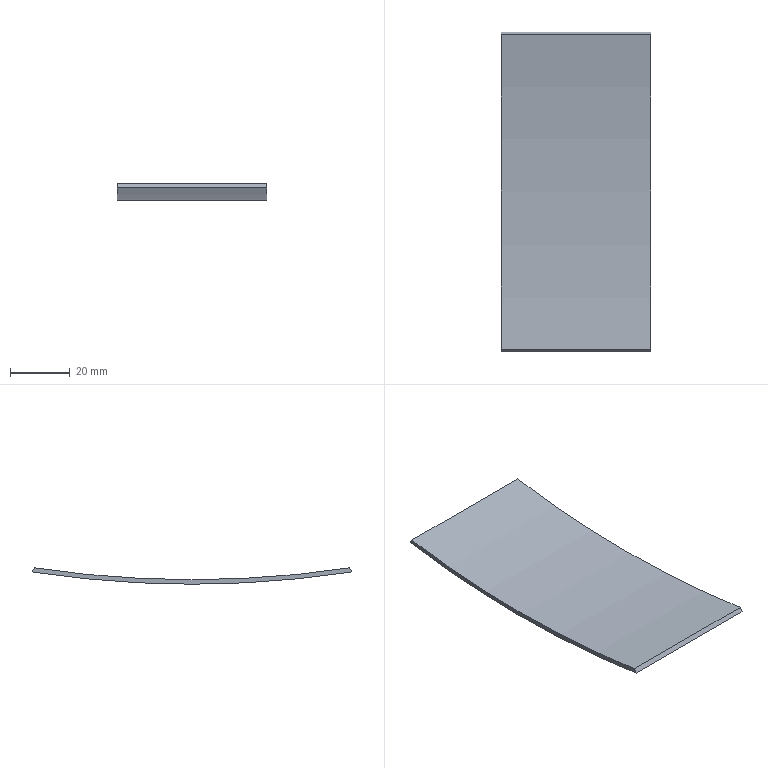Part | STEP file | 1 solid | 6 faces | box 50 x 106.693 x 5.46 mm | volume 7969 mm3 | plane 4 | cylinder 2 | commonest cylinder face diameters 700 x1 703 x1
STEP:
#1=CARTESIAN_POINT('',(0.,0.,0.));
#2=DIRECTION('',(0.,0.,1.));
#3=DIRECTION('',(1.,0.,0.));
#4=AXIS2_PLACEMENT_3D('',#1,#2,#3);
#5=CARTESIAN_POINT('',(25.,53.346,-347.428));
#6=VERTEX_POINT('',#5);
#7=CARTESIAN_POINT('',(25.,-53.346,-347.428));
#8=VERTEX_POINT('',#7);
#9=CARTESIAN_POINT('',(25.,0.,0.));
#10=DIRECTION('',(-1.,0.,0.));
#11=DIRECTION('',(0.,0.,-1.));
#12=AXIS2_PLACEMENT_3D('',#9,#10,#11);
#13=CIRCLE('',#12,351.5);
#14=CARTESIAN_POINT('',(-25.,0.,0.));
#15=DIRECTION('',(1.,0.,0.));
#16=DIRECTION('',(0.,0.,-1.));
#17=AXIS2_PLACEMENT_3D('',#14,#15,#16);
#18=CYLINDRICAL_SURFACE('',#17,351.5);
#19=CARTESIAN_POINT('',(6.283,50.));
#20=DIRECTION('',(-1.,0.));
#21=VECTOR('',#20,1.);
#22=LINE('',#19,#21);
#23=(GEOMETRIC_REPRESENTATION_CONTEXT(2)PARAMETRIC_REPRESENTATION_CONTEXT()REPRESENTATION_CONTEXT('',''));
#24=DEFINITIONAL_REPRESENTATION('',(#22),#23);
#25=PCURVE('',#18,#24);
#26=CARTESIAN_POINT('',(25.,-69.931,-393.84));
#27=DIRECTION('',(1.,0.,0.));
#28=DIRECTION('',(0.,0.,-1.));
#29=AXIS2_PLACEMENT_3D('',#26,#27,#28);
#30=PLANE('',#29);
#31=CARTESIAN_POINT('',(-42.34,69.931));
#32=CARTESIAN_POINT('',(-42.34,-538.885));
#33=CARTESIAN_POINT('',(-569.59,-234.477));
#34=CARTESIAN_POINT('',(-1096.84,69.931));
#35=CARTESIAN_POINT('',(-569.59,374.339));
#36=CARTESIAN_POINT('',(-42.34,678.747));
#37=CARTESIAN_POINT('',(-42.34,69.931));
#38=(BOUNDED_CURVE()B_SPLINE_CURVE(2,(#31,#32,#33,#34,#35,#36,#37),.UNSPECIFIED.,.T.,.F.)B_SPLINE_CURVE_WITH_KNOTS((1,2,2,2,2,1),(-2.094,0.,2.094,4.189,6.283,8.378),.UNSPECIFIED.)CURVE()GEOMETRIC_REPRESENTATION_ITEM()RATIONAL_B_SPLINE_CURVE((1.,0.5,1.,0.5,1.,0.5,1.))REPRESENTATION_ITEM(''));
#39=(GEOMETRIC_REPRESENTATION_CONTEXT(2)PARAMETRIC_REPRESENTATION_CONTEXT()REPRESENTATION_CONTEXT('',''));
#40=DEFINITIONAL_REPRESENTATION('',(#38),#39);
#41=PCURVE('',#30,#40);
#42=SURFACE_CURVE('',#13,(#25,#41),.PCURVE_S1.);
#43=EDGE_CURVE('',#6,#8,#42,.T.);
#44=ORIENTED_EDGE('',*,*,#43,.T.);
#45=CARTESIAN_POINT('',(-25.,-53.346,-347.428));
#46=VERTEX_POINT('',#45);
#47=CARTESIAN_POINT('',(-25.,-53.346,-347.428));
#48=DIRECTION('',(-1.,0.,0.));
#49=VECTOR('',#48,1.);
#50=LINE('',#47,#49);
#51=CARTESIAN_POINT('',(-0.1524,0.));
#52=DIRECTION('',(0.,-1.));
#53=VECTOR('',#52,1.);
#54=LINE('',#51,#53);
#55=(GEOMETRIC_REPRESENTATION_CONTEXT(2)PARAMETRIC_REPRESENTATION_CONTEXT()REPRESENTATION_CONTEXT('',''));
#56=DEFINITIONAL_REPRESENTATION('',(#54),#55);
#57=PCURVE('',#18,#56);
#58=CARTESIAN_POINT('',(-25.,-52.5,-346.04));
#59=DIRECTION('',(0.,0.8538,-0.5206));
#60=DIRECTION('',(0.,0.5206,0.8538));
#61=AXIS2_PLACEMENT_3D('',#58,#59,#60);
#62=PLANE('',#61);
#63=CARTESIAN_POINT('',(-1.626,0.));
#64=DIRECTION('',(0.,-1.));
#65=VECTOR('',#64,1.);
#66=LINE('',#63,#65);
#67=(GEOMETRIC_REPRESENTATION_CONTEXT(2)PARAMETRIC_REPRESENTATION_CONTEXT()REPRESENTATION_CONTEXT('',''));
#68=DEFINITIONAL_REPRESENTATION('',(#66),#67);
#69=PCURVE('',#62,#68);
#70=SURFACE_CURVE('',#50,(#57,#69),.PCURVE_S1.);
#71=EDGE_CURVE('',#8,#46,#70,.T.);
#72=ORIENTED_EDGE('',*,*,#71,.T.);
#73=CARTESIAN_POINT('',(-25.,53.346,-347.428));
#74=VERTEX_POINT('',#73);
#75=CARTESIAN_POINT('',(-25.,0.,0.));
#76=DIRECTION('',(1.,0.,0.));
#77=DIRECTION('',(0.,0.,-1.));
#78=AXIS2_PLACEMENT_3D('',#75,#76,#77);
#79=CIRCLE('',#78,351.5);
#80=CARTESIAN_POINT('',(-6.283,0.));
#81=DIRECTION('',(1.,0.));
#82=VECTOR('',#81,1.);
#83=LINE('',#80,#82);
#84=(GEOMETRIC_REPRESENTATION_CONTEXT(2)PARAMETRIC_REPRESENTATION_CONTEXT()REPRESENTATION_CONTEXT('',''));
#85=DEFINITIONAL_REPRESENTATION('',(#83),#84);
#86=PCURVE('',#18,#85);
#87=CARTESIAN_POINT('',(-25.,0.,0.));
#88=DIRECTION('',(-1.,0.,0.));
#89=DIRECTION('',(0.,0.,1.));
#90=AXIS2_PLACEMENT_3D('',#87,#88,#89);
#91=PLANE('',#90);
#92=CARTESIAN_POINT('',(-351.5,0.));
#93=CARTESIAN_POINT('',(-351.5,608.816));
#94=CARTESIAN_POINT('',(175.75,304.408));
#95=CARTESIAN_POINT('',(703.,0.));
#96=CARTESIAN_POINT('',(175.75,-304.408));
#97=CARTESIAN_POINT('',(-351.5,-608.816));
#98=CARTESIAN_POINT('',(-351.5,0.));
#99=(BOUNDED_CURVE()B_SPLINE_CURVE(2,(#92,#93,#94,#95,#96,#97,#98),.UNSPECIFIED.,.T.,.F.)B_SPLINE_CURVE_WITH_KNOTS((1,2,2,2,2,1),(-2.094,0.,2.094,4.189,6.283,8.378),.UNSPECIFIED.)CURVE()GEOMETRIC_REPRESENTATION_ITEM()RATIONAL_B_SPLINE_CURVE((1.,0.5,1.,0.5,1.,0.5,1.))REPRESENTATION_ITEM(''));
#100=(GEOMETRIC_REPRESENTATION_CONTEXT(2)PARAMETRIC_REPRESENTATION_CONTEXT()REPRESENTATION_CONTEXT('',''));
#101=DEFINITIONAL_REPRESENTATION('',(#99),#100);
#102=PCURVE('',#91,#101);
#103=SURFACE_CURVE('',#79,(#86,#102),.PCURVE_S1.);
#104=EDGE_CURVE('',#46,#74,#103,.T.);
#105=ORIENTED_EDGE('',*,*,#104,.T.);
#106=CARTESIAN_POINT('',(-25.,53.346,-347.428));
#107=DIRECTION('',(1.,0.,0.));
#108=VECTOR('',#107,1.);
#109=LINE('',#106,#108);
#110=CARTESIAN_POINT('',(0.1524,0.));
#111=DIRECTION('',(0.,1.));
#112=VECTOR('',#111,1.);
#113=LINE('',#110,#112);
#114=(GEOMETRIC_REPRESENTATION_CONTEXT(2)PARAMETRIC_REPRESENTATION_CONTEXT()REPRESENTATION_CONTEXT('',''));
#115=DEFINITIONAL_REPRESENTATION('',(#113),#114);
#116=PCURVE('',#18,#115);
#117=CARTESIAN_POINT('',(-25.,53.346,-347.428));
#118=DIRECTION('',(0.,-0.8538,-0.5206));
#119=DIRECTION('',(0.,0.5206,-0.8538));
#120=AXIS2_PLACEMENT_3D('',#117,#118,#119);
#121=PLANE('',#120);
#122=CARTESIAN_POINT('',(0.,0.));
#123=DIRECTION('',(0.,1.));
#124=VECTOR('',#123,1.);
#125=LINE('',#122,#124);
#126=(GEOMETRIC_REPRESENTATION_CONTEXT(2)PARAMETRIC_REPRESENTATION_CONTEXT()REPRESENTATION_CONTEXT('',''));
#127=DEFINITIONAL_REPRESENTATION('',(#125),#126);
#128=PCURVE('',#121,#127);
#129=SURFACE_CURVE('',#109,(#116,#128),.PCURVE_S1.);
#130=EDGE_CURVE('',#74,#6,#129,.T.);
#131=ORIENTED_EDGE('',*,*,#130,.T.);
#132=EDGE_LOOP('',(#44,#72,#105,#131));
#133=FACE_BOUND('',#132,.T.);
#134=ADVANCED_FACE('',(#133),#18,.T.);
#135=ORIENTED_EDGE('',*,*,#71,.F.);
#136=CARTESIAN_POINT('',(25.,-52.5,-346.04));
#137=VERTEX_POINT('',#136);
#138=CARTESIAN_POINT('',(25.,-52.5,-346.04));
#139=DIRECTION('',(0.,-0.5206,-0.8538));
#140=VECTOR('',#139,1.);
#141=LINE('',#138,#140);
#142=CARTESIAN_POINT('',(0.,50.));
#143=DIRECTION('',(-1.,0.));
#144=VECTOR('',#143,1.);
#145=LINE('',#142,#144);
#146=(GEOMETRIC_REPRESENTATION_CONTEXT(2)PARAMETRIC_REPRESENTATION_CONTEXT()REPRESENTATION_CONTEXT('',''));
#147=DEFINITIONAL_REPRESENTATION('',(#145),#146);
#148=PCURVE('',#62,#147);
#149=CARTESIAN_POINT('',(-47.799,17.431));
#150=DIRECTION('',(0.8538,-0.5206));
#151=VECTOR('',#150,1.);
#152=LINE('',#149,#151);
#153=(GEOMETRIC_REPRESENTATION_CONTEXT(2)PARAMETRIC_REPRESENTATION_CONTEXT()REPRESENTATION_CONTEXT('',''));
#154=DEFINITIONAL_REPRESENTATION('',(#152),#153);
#155=PCURVE('',#30,#154);
#156=SURFACE_CURVE('',#141,(#148,#155),.PCURVE_S1.);
#157=EDGE_CURVE('',#137,#8,#156,.T.);
#158=ORIENTED_EDGE('',*,*,#157,.F.);
#159=CARTESIAN_POINT('',(-25.,-52.5,-346.04));
#160=VERTEX_POINT('',#159);
#161=CARTESIAN_POINT('',(-25.,-52.5,-346.04));
#162=DIRECTION('',(1.,0.,0.));
#163=VECTOR('',#162,1.);
#164=LINE('',#161,#163);
#165=CARTESIAN_POINT('',(0.,0.));
#166=DIRECTION('',(0.,1.));
#167=VECTOR('',#166,1.);
#168=LINE('',#165,#167);
#169=(GEOMETRIC_REPRESENTATION_CONTEXT(2)PARAMETRIC_REPRESENTATION_CONTEXT()REPRESENTATION_CONTEXT('',''));
#170=DEFINITIONAL_REPRESENTATION('',(#168),#169);
#171=PCURVE('',#62,#170);
#172=CARTESIAN_POINT('',(-25.,0.,0.));
#173=DIRECTION('',(1.,0.,0.));
#174=DIRECTION('',(0.,0.,-1.));
#175=AXIS2_PLACEMENT_3D('',#172,#173,#174);
#176=CYLINDRICAL_SURFACE('',#175,350.);
#177=CARTESIAN_POINT('',(-0.1506,0.));
#178=DIRECTION('',(0.,1.));
#179=VECTOR('',#178,1.);
#180=LINE('',#177,#179);
#181=(GEOMETRIC_REPRESENTATION_CONTEXT(2)PARAMETRIC_REPRESENTATION_CONTEXT()REPRESENTATION_CONTEXT('',''));
#182=DEFINITIONAL_REPRESENTATION('',(#180),#181);
#183=PCURVE('',#176,#182);
#184=SURFACE_CURVE('',#164,(#171,#183),.PCURVE_S1.);
#185=EDGE_CURVE('',#160,#137,#184,.T.);
#186=ORIENTED_EDGE('',*,*,#185,.F.);
#187=CARTESIAN_POINT('',(-25.,-52.5,-346.04));
#188=DIRECTION('',(0.,0.5206,0.8538));
#189=VECTOR('',#188,1.);
#190=LINE('',#187,#189);
#191=CARTESIAN_POINT('',(0.,0.));
#192=DIRECTION('',(1.,0.));
#193=VECTOR('',#192,1.);
#194=LINE('',#191,#193);
#195=(GEOMETRIC_REPRESENTATION_CONTEXT(2)PARAMETRIC_REPRESENTATION_CONTEXT()REPRESENTATION_CONTEXT('',''));
#196=DEFINITIONAL_REPRESENTATION('',(#194),#195);
#197=PCURVE('',#62,#196);
#198=CARTESIAN_POINT('',(-346.04,-52.5));
#199=DIRECTION('',(0.8538,0.5206));
#200=VECTOR('',#199,1.);
#201=LINE('',#198,#200);
#202=(GEOMETRIC_REPRESENTATION_CONTEXT(2)PARAMETRIC_REPRESENTATION_CONTEXT()REPRESENTATION_CONTEXT('',''));
#203=DEFINITIONAL_REPRESENTATION('',(#201),#202);
#204=PCURVE('',#91,#203);
#205=SURFACE_CURVE('',#190,(#197,#204),.PCURVE_S1.);
#206=EDGE_CURVE('',#46,#160,#205,.T.);
#207=ORIENTED_EDGE('',*,*,#206,.F.);
#208=EDGE_LOOP('',(#135,#158,#186,#207));
#209=FACE_BOUND('',#208,.T.);
#210=ADVANCED_FACE('',(#209),#62,.F.);
#211=ORIENTED_EDGE('',*,*,#157,.T.);
#212=ORIENTED_EDGE('',*,*,#43,.F.);
#213=CARTESIAN_POINT('',(25.,52.5,-346.04));
#214=VERTEX_POINT('',#213);
#215=CARTESIAN_POINT('',(25.,53.346,-347.428));
#216=DIRECTION('',(0.,-0.5206,0.8538));
#217=VECTOR('',#216,1.);
#218=LINE('',#215,#217);
#219=CARTESIAN_POINT('',(-46.411,123.278));
#220=DIRECTION('',(-0.8538,-0.5206));
#221=VECTOR('',#220,1.);
#222=LINE('',#219,#221);
#223=(GEOMETRIC_REPRESENTATION_CONTEXT(2)PARAMETRIC_REPRESENTATION_CONTEXT()REPRESENTATION_CONTEXT('',''));
#224=DEFINITIONAL_REPRESENTATION('',(#222),#223);
#225=PCURVE('',#30,#224);
#226=CARTESIAN_POINT('',(0.,50.));
#227=DIRECTION('',(-1.,0.));
#228=VECTOR('',#227,1.);
#229=LINE('',#226,#228);
#230=(GEOMETRIC_REPRESENTATION_CONTEXT(2)PARAMETRIC_REPRESENTATION_CONTEXT()REPRESENTATION_CONTEXT('',''));
#231=DEFINITIONAL_REPRESENTATION('',(#229),#230);
#232=PCURVE('',#121,#231);
#233=SURFACE_CURVE('',#218,(#225,#232),.PCURVE_S1.);
#234=EDGE_CURVE('',#6,#214,#233,.T.);
#235=ORIENTED_EDGE('',*,*,#234,.T.);
#236=CARTESIAN_POINT('',(25.,0.,0.));
#237=DIRECTION('',(-1.,0.,0.));
#238=DIRECTION('',(0.,0.,-1.));
#239=AXIS2_PLACEMENT_3D('',#236,#237,#238);
#240=CIRCLE('',#239,350.);
#241=CARTESIAN_POINT('',(-43.84,69.931));
#242=CARTESIAN_POINT('',(-43.84,-536.286));
#243=CARTESIAN_POINT('',(-568.84,-233.178));
#244=CARTESIAN_POINT('',(-1093.84,69.931));
#245=CARTESIAN_POINT('',(-568.84,373.04));
#246=CARTESIAN_POINT('',(-43.84,676.149));
#247=CARTESIAN_POINT('',(-43.84,69.931));
#248=(BOUNDED_CURVE()B_SPLINE_CURVE(2,(#241,#242,#243,#244,#245,#246,#247),.UNSPECIFIED.,.T.,.F.)B_SPLINE_CURVE_WITH_KNOTS((1,2,2,2,2,1),(-2.094,0.,2.094,4.189,6.283,8.378),.UNSPECIFIED.)CURVE()GEOMETRIC_REPRESENTATION_ITEM()RATIONAL_B_SPLINE_CURVE((1.,0.5,1.,0.5,1.,0.5,1.))REPRESENTATION_ITEM(''));
#249=(GEOMETRIC_REPRESENTATION_CONTEXT(2)PARAMETRIC_REPRESENTATION_CONTEXT()REPRESENTATION_CONTEXT('',''));
#250=DEFINITIONAL_REPRESENTATION('',(#248),#249);
#251=PCURVE('',#30,#250);
#252=CARTESIAN_POINT('',(6.283,50.));
#253=DIRECTION('',(-1.,0.));
#254=VECTOR('',#253,1.);
#255=LINE('',#252,#254);
#256=(GEOMETRIC_REPRESENTATION_CONTEXT(2)PARAMETRIC_REPRESENTATION_CONTEXT()REPRESENTATION_CONTEXT('',''));
#257=DEFINITIONAL_REPRESENTATION('',(#255),#256);
#258=PCURVE('',#176,#257);
#259=SURFACE_CURVE('',#240,(#251,#258),.PCURVE_S1.);
#260=EDGE_CURVE('',#214,#137,#259,.T.);
#261=ORIENTED_EDGE('',*,*,#260,.T.);
#262=EDGE_LOOP('',(#211,#212,#235,#261));
#263=FACE_BOUND('',#262,.T.);
#264=ADVANCED_FACE('',(#263),#30,.T.);
#265=CARTESIAN_POINT('',(-25.,52.5,-346.04));
#266=VERTEX_POINT('',#265);
#267=CARTESIAN_POINT('',(-25.,0.,0.));
#268=DIRECTION('',(1.,0.,0.));
#269=DIRECTION('',(0.,0.,-1.));
#270=AXIS2_PLACEMENT_3D('',#267,#268,#269);
#271=CIRCLE('',#270,350.);
#272=CARTESIAN_POINT('',(-350.,0.));
#273=CARTESIAN_POINT('',(-350.,606.218));
#274=CARTESIAN_POINT('',(175.,303.109));
#275=CARTESIAN_POINT('',(700.,0.));
#276=CARTESIAN_POINT('',(175.,-303.109));
#277=CARTESIAN_POINT('',(-350.,-606.218));
#278=CARTESIAN_POINT('',(-350.,0.));
#279=(BOUNDED_CURVE()B_SPLINE_CURVE(2,(#272,#273,#274,#275,#276,#277,#278),.UNSPECIFIED.,.T.,.F.)B_SPLINE_CURVE_WITH_KNOTS((1,2,2,2,2,1),(-2.094,0.,2.094,4.189,6.283,8.378),.UNSPECIFIED.)CURVE()GEOMETRIC_REPRESENTATION_ITEM()RATIONAL_B_SPLINE_CURVE((1.,0.5,1.,0.5,1.,0.5,1.))REPRESENTATION_ITEM(''));
#280=(GEOMETRIC_REPRESENTATION_CONTEXT(2)PARAMETRIC_REPRESENTATION_CONTEXT()REPRESENTATION_CONTEXT('',''));
#281=DEFINITIONAL_REPRESENTATION('',(#279),#280);
#282=PCURVE('',#91,#281);
#283=CARTESIAN_POINT('',(-6.283,0.));
#284=DIRECTION('',(1.,0.));
#285=VECTOR('',#284,1.);
#286=LINE('',#283,#285);
#287=(GEOMETRIC_REPRESENTATION_CONTEXT(2)PARAMETRIC_REPRESENTATION_CONTEXT()REPRESENTATION_CONTEXT('',''));
#288=DEFINITIONAL_REPRESENTATION('',(#286),#287);
#289=PCURVE('',#176,#288);
#290=SURFACE_CURVE('',#271,(#282,#289),.PCURVE_S1.);
#291=EDGE_CURVE('',#160,#266,#290,.T.);
#292=ORIENTED_EDGE('',*,*,#291,.T.);
#293=CARTESIAN_POINT('',(-25.,52.5,-346.04));
#294=DIRECTION('',(0.,0.5206,-0.8538));
#295=VECTOR('',#294,1.);
#296=LINE('',#293,#295);
#297=CARTESIAN_POINT('',(-346.04,52.5));
#298=DIRECTION('',(-0.8538,0.5206));
#299=VECTOR('',#298,1.);
#300=LINE('',#297,#299);
#301=(GEOMETRIC_REPRESENTATION_CONTEXT(2)PARAMETRIC_REPRESENTATION_CONTEXT()REPRESENTATION_CONTEXT('',''));
#302=DEFINITIONAL_REPRESENTATION('',(#300),#301);
#303=PCURVE('',#91,#302);
#304=CARTESIAN_POINT('',(-1.626,0.));
#305=DIRECTION('',(1.,0.));
#306=VECTOR('',#305,1.);
#307=LINE('',#304,#306);
#308=(GEOMETRIC_REPRESENTATION_CONTEXT(2)PARAMETRIC_REPRESENTATION_CONTEXT()REPRESENTATION_CONTEXT('',''));
#309=DEFINITIONAL_REPRESENTATION('',(#307),#308);
#310=PCURVE('',#121,#309);
#311=SURFACE_CURVE('',#296,(#303,#310),.PCURVE_S1.);
#312=EDGE_CURVE('',#266,#74,#311,.T.);
#313=ORIENTED_EDGE('',*,*,#312,.T.);
#314=ORIENTED_EDGE('',*,*,#104,.F.);
#315=ORIENTED_EDGE('',*,*,#206,.T.);
#316=EDGE_LOOP('',(#292,#313,#314,#315));
#317=FACE_BOUND('',#316,.T.);
#318=ADVANCED_FACE('',(#317),#91,.T.);
#319=CARTESIAN_POINT('',(-25.,52.5,-346.04));
#320=DIRECTION('',(1.,0.,0.));
#321=VECTOR('',#320,1.);
#322=LINE('',#319,#321);
#323=CARTESIAN_POINT('',(0.1506,0.));
#324=DIRECTION('',(0.,1.));
#325=VECTOR('',#324,1.);
#326=LINE('',#323,#325);
#327=(GEOMETRIC_REPRESENTATION_CONTEXT(2)PARAMETRIC_REPRESENTATION_CONTEXT()REPRESENTATION_CONTEXT('',''));
#328=DEFINITIONAL_REPRESENTATION('',(#326),#327);
#329=PCURVE('',#176,#328);
#330=CARTESIAN_POINT('',(-1.626,0.));
#331=DIRECTION('',(0.,1.));
#332=VECTOR('',#331,1.);
#333=LINE('',#330,#332);
#334=(GEOMETRIC_REPRESENTATION_CONTEXT(2)PARAMETRIC_REPRESENTATION_CONTEXT()REPRESENTATION_CONTEXT('',''));
#335=DEFINITIONAL_REPRESENTATION('',(#333),#334);
#336=PCURVE('',#121,#335);
#337=SURFACE_CURVE('',#322,(#329,#336),.PCURVE_S1.);
#338=EDGE_CURVE('',#266,#214,#337,.T.);
#339=ORIENTED_EDGE('',*,*,#338,.T.);
#340=ORIENTED_EDGE('',*,*,#260,.T.);
#341=ORIENTED_EDGE('',*,*,#185,.F.);
#342=ORIENTED_EDGE('',*,*,#291,.T.);
#343=EDGE_LOOP('',(#339,#340,#341,#342));
#344=FACE_BOUND('',#343,.F.);
#345=ADVANCED_FACE('',(#344),#176,.F.);
#346=ORIENTED_EDGE('',*,*,#338,.T.);
#347=ORIENTED_EDGE('',*,*,#234,.F.);
#348=ORIENTED_EDGE('',*,*,#130,.F.);
#349=ORIENTED_EDGE('',*,*,#312,.F.);
#350=EDGE_LOOP('',(#346,#347,#348,#349));
#351=FACE_BOUND('',#350,.T.);
#352=ADVANCED_FACE('',(#351),#121,.F.);
#353=CLOSED_SHELL('',(#134,#210,#264,#318,#345,#352));
#354=MANIFOLD_SOLID_BREP('',#353);
#355=(LENGTH_UNIT()NAMED_UNIT(*)SI_UNIT(.MILLI.,.METRE.));
#356=UNCERTAINTY_MEASURE_WITH_UNIT(LENGTH_MEASURE(0.0000001),#355,'','');
#357=(NAMED_UNIT(*)PLANE_ANGLE_UNIT()SI_UNIT($,.RADIAN.));
#358=(NAMED_UNIT(*)SI_UNIT($,.STERADIAN.)SOLID_ANGLE_UNIT());
#359=(GEOMETRIC_REPRESENTATION_CONTEXT(3)GLOBAL_UNCERTAINTY_ASSIGNED_CONTEXT((#356))GLOBAL_UNIT_ASSIGNED_CONTEXT((#355,#357,#358))REPRESENTATION_CONTEXT('',''));
#360=ADVANCED_BREP_SHAPE_REPRESENTATION('',(#4,#354),#359);